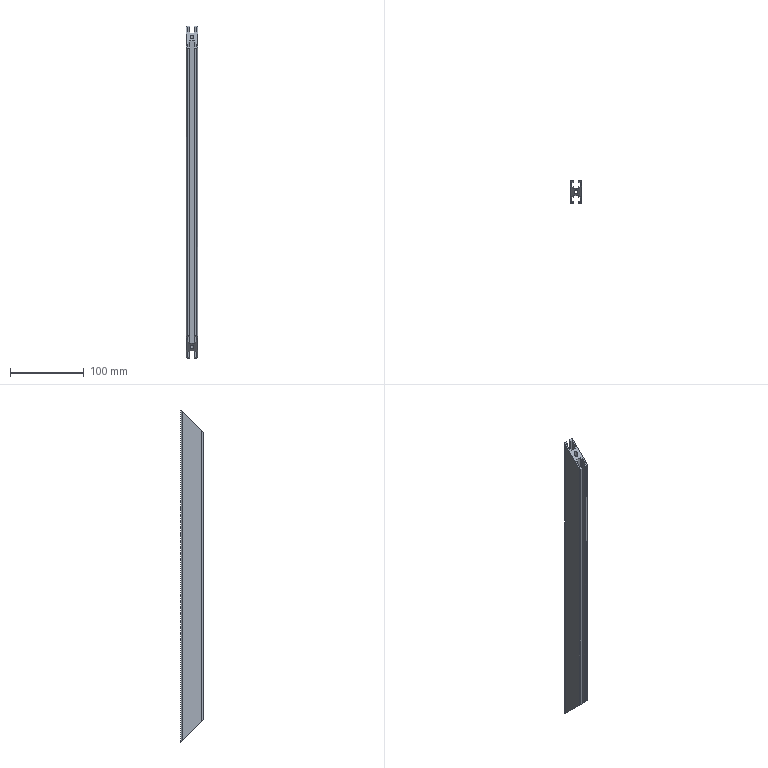Part | STEP file | OB1530-450 | 1 solid | 36 faces | box 15 x 30 x 450 mm | volume 102663 mm3 | plane 30 | cylinder 6 | commonest cylinder face diameters 3 x4 5 x2
STEP:
#1=CARTESIAN_POINT('',(2.5,0.,435.));
#2=VERTEX_POINT('',#1);
#3=CARTESIAN_POINT('',(-2.5,0.,435.));
#4=VERTEX_POINT('',#3);
#5=CARTESIAN_POINT('',(2.5,0.,435.));
#6=CARTESIAN_POINT('',(2.5,-5.,430.));
#7=CARTESIAN_POINT('',(-2.5,-5.,430.));
#8=CARTESIAN_POINT('',(-2.5,0.,435.));
#9=(BOUNDED_CURVE()B_SPLINE_CURVE(3,(#5,#6,#7,#8),.UNSPECIFIED.,.F.,.F.)B_SPLINE_CURVE_WITH_KNOTS((4,4),(4.712,7.854),.UNSPECIFIED.)CURVE()GEOMETRIC_REPRESENTATION_ITEM()RATIONAL_B_SPLINE_CURVE((1.,0.3333,0.3333,1.))REPRESENTATION_ITEM(''));
#10=EDGE_CURVE('',#2,#4,#9,.T.);
#11=ORIENTED_EDGE('',*,*,#10,.F.);
#12=CARTESIAN_POINT('',(2.5,0.,15.));
#13=VERTEX_POINT('',#12);
#14=CARTESIAN_POINT('',(2.5,0.,450.));
#15=DIRECTION('',(0.,0.,-1.));
#16=VECTOR('',#15,1000.);
#17=LINE('',#14,#16);
#18=EDGE_CURVE('',#2,#13,#17,.T.);
#19=ORIENTED_EDGE('',*,*,#18,.T.);
#20=CARTESIAN_POINT('',(-2.5,0.,15.));
#21=VERTEX_POINT('',#20);
#22=CARTESIAN_POINT('',(-2.5,0.,15.));
#23=CARTESIAN_POINT('',(-2.5,-5.,20.));
#24=CARTESIAN_POINT('',(2.5,-5.,20.));
#25=CARTESIAN_POINT('',(2.5,0.,15.));
#26=(BOUNDED_CURVE()B_SPLINE_CURVE(3,(#22,#23,#24,#25),.UNSPECIFIED.,.F.,.F.)B_SPLINE_CURVE_WITH_KNOTS((4,4),(1.571,4.712),.UNSPECIFIED.)CURVE()GEOMETRIC_REPRESENTATION_ITEM()RATIONAL_B_SPLINE_CURVE((1.,0.3333,0.3333,1.))REPRESENTATION_ITEM(''));
#27=EDGE_CURVE('',#21,#13,#26,.T.);
#28=ORIENTED_EDGE('',*,*,#27,.F.);
#29=CARTESIAN_POINT('',(-2.5,0.,450.));
#30=DIRECTION('',(0.,0.,-1.));
#31=VECTOR('',#30,1000.);
#32=LINE('',#29,#31);
#33=EDGE_CURVE('',#4,#21,#32,.T.);
#34=ORIENTED_EDGE('',*,*,#33,.F.);
#35=EDGE_LOOP('',(#11,#19,#28,#34));
#36=FACE_OUTER_BOUND('',#35,.T.);
#37=CARTESIAN_POINT('',(0.,0.,450.));
#38=DIRECTION('',(0.,0.,-1.));
#39=DIRECTION('',(-1.,0.,0.));
#40=AXIS2_PLACEMENT_3D('',#37,#38,#39);
#41=CYLINDRICAL_SURFACE('',#40,2.5);
#42=ADVANCED_FACE('',(#36),#41,.F.);
#43=CARTESIAN_POINT('',(6.,15.,450.));
#44=VERTEX_POINT('',#43);
#45=CARTESIAN_POINT('',(6.,15.,0.));
#46=VERTEX_POINT('',#45);
#47=CARTESIAN_POINT('',(6.,15.,450.));
#48=DIRECTION('',(0.,0.,-1.));
#49=VECTOR('',#48,1000.);
#50=LINE('',#47,#49);
#51=EDGE_CURVE('',#44,#46,#50,.T.);
#52=ORIENTED_EDGE('',*,*,#51,.F.);
#53=CARTESIAN_POINT('',(7.5,13.5,448.5));
#54=VERTEX_POINT('',#53);
#55=CARTESIAN_POINT('',(6.,15.,450.));
#56=CARTESIAN_POINT('',(6.879,15.,450.));
#57=CARTESIAN_POINT('',(7.5,14.379,449.379));
#58=CARTESIAN_POINT('',(7.5,13.5,448.5));
#59=(BOUNDED_CURVE()B_SPLINE_CURVE(3,(#55,#56,#57,#58),.UNSPECIFIED.,.F.,.F.)B_SPLINE_CURVE_WITH_KNOTS((4,4),(3.142,4.712),.UNSPECIFIED.)CURVE()GEOMETRIC_REPRESENTATION_ITEM()RATIONAL_B_SPLINE_CURVE((1.,0.8047,0.8047,1.))REPRESENTATION_ITEM(''));
#60=EDGE_CURVE('',#44,#54,#59,.T.);
#61=ORIENTED_EDGE('',*,*,#60,.T.);
#62=CARTESIAN_POINT('',(7.5,13.5,1.5));
#63=VERTEX_POINT('',#62);
#64=CARTESIAN_POINT('',(7.5,13.5,450.));
#65=DIRECTION('',(0.,0.,-1.));
#66=VECTOR('',#65,1000.);
#67=LINE('',#64,#66);
#68=EDGE_CURVE('',#54,#63,#67,.T.);
#69=ORIENTED_EDGE('',*,*,#68,.T.);
#70=CARTESIAN_POINT('',(7.5,13.5,1.5));
#71=CARTESIAN_POINT('',(7.5,14.379,0.6213));
#72=CARTESIAN_POINT('',(6.879,15.,0.));
#73=CARTESIAN_POINT('',(6.,15.,0.));
#74=(BOUNDED_CURVE()B_SPLINE_CURVE(3,(#70,#71,#72,#73),.UNSPECIFIED.,.F.,.F.)B_SPLINE_CURVE_WITH_KNOTS((4,4),(4.712,6.283),.UNSPECIFIED.)CURVE()GEOMETRIC_REPRESENTATION_ITEM()RATIONAL_B_SPLINE_CURVE((1.,0.8047,0.8047,1.))REPRESENTATION_ITEM(''));
#75=EDGE_CURVE('',#63,#46,#74,.T.);
#76=ORIENTED_EDGE('',*,*,#75,.T.);
#77=EDGE_LOOP('',(#52,#61,#69,#76));
#78=FACE_OUTER_BOUND('',#77,.T.);
#79=CARTESIAN_POINT('',(6.,13.5,450.));
#80=DIRECTION('',(0.,0.,-1.));
#81=DIRECTION('',(-1.,0.,0.));
#82=AXIS2_PLACEMENT_3D('',#79,#80,#81);
#83=CYLINDRICAL_SURFACE('',#82,1.5);
#84=ADVANCED_FACE('',(#78),#83,.T.);
#85=CARTESIAN_POINT('',(3.25,15.,0.));
#86=VERTEX_POINT('',#85);
#87=CARTESIAN_POINT('',(6.,15.,0.));
#88=DIRECTION('',(-1.,0.,0.));
#89=VECTOR('',#88,1000.);
#90=LINE('',#87,#89);
#91=EDGE_CURVE('',#46,#86,#90,.T.);
#92=ORIENTED_EDGE('',*,*,#91,.T.);
#93=CARTESIAN_POINT('',(3.25,15.,450.));
#94=VERTEX_POINT('',#93);
#95=CARTESIAN_POINT('',(3.25,15.,450.));
#96=DIRECTION('',(0.,0.,-1.));
#97=VECTOR('',#96,1000.);
#98=LINE('',#95,#97);
#99=EDGE_CURVE('',#94,#86,#98,.T.);
#100=ORIENTED_EDGE('',*,*,#99,.F.);
#101=CARTESIAN_POINT('',(6.,15.,450.));
#102=DIRECTION('',(-1.,0.,0.));
#103=VECTOR('',#102,1000.);
#104=LINE('',#101,#103);
#105=EDGE_CURVE('',#44,#94,#104,.T.);
#106=ORIENTED_EDGE('',*,*,#105,.F.);
#107=ORIENTED_EDGE('',*,*,#51,.T.);
#108=EDGE_LOOP('',(#92,#100,#106,#107));
#109=FACE_OUTER_BOUND('',#108,.T.);
#110=CARTESIAN_POINT('',(6.,15.,450.));
#111=DIRECTION('',(0.,-1.,0.));
#112=DIRECTION('',(0.,0.,-1.));
#113=AXIS2_PLACEMENT_3D('',#110,#111,#112);
#114=PLANE('',#113);
#115=ADVANCED_FACE('',(#109),#114,.F.);
#116=CARTESIAN_POINT('',(3.25,13.,448.));
#117=VERTEX_POINT('',#116);
#118=CARTESIAN_POINT('',(3.25,13.,2.));
#119=VERTEX_POINT('',#118);
#120=CARTESIAN_POINT('',(3.25,13.,450.));
#121=DIRECTION('',(0.,0.,-1.));
#122=VECTOR('',#121,1000.);
#123=LINE('',#120,#122);
#124=EDGE_CURVE('',#117,#119,#123,.T.);
#125=ORIENTED_EDGE('',*,*,#124,.F.);
#126=CARTESIAN_POINT('',(3.25,15.,450.));
#127=DIRECTION('',(0.,0.7071,0.7071));
#128=VECTOR('',#127,1000.);
#129=LINE('',#126,#128);
#130=EDGE_CURVE('',#117,#94,#129,.T.);
#131=ORIENTED_EDGE('',*,*,#130,.T.);
#132=ORIENTED_EDGE('',*,*,#99,.T.);
#133=CARTESIAN_POINT('',(3.25,-210.,225.));
#134=DIRECTION('',(0.,-0.7071,0.7071));
#135=VECTOR('',#134,1000.);
#136=LINE('',#133,#135);
#137=EDGE_CURVE('',#86,#119,#136,.T.);
#138=ORIENTED_EDGE('',*,*,#137,.T.);
#139=EDGE_LOOP('',(#125,#131,#132,#138));
#140=FACE_OUTER_BOUND('',#139,.T.);
#141=CARTESIAN_POINT('',(3.25,15.,450.));
#142=DIRECTION('',(1.,0.,0.));
#143=DIRECTION('',(0.,0.,-1.));
#144=AXIS2_PLACEMENT_3D('',#141,#142,#143);
#145=PLANE('',#144);
#146=ADVANCED_FACE('',(#140),#145,.F.);
#147=CARTESIAN_POINT('',(5.5,13.,448.));
#148=VERTEX_POINT('',#147);
#149=CARTESIAN_POINT('',(5.5,13.,2.));
#150=VERTEX_POINT('',#149);
#151=CARTESIAN_POINT('',(5.5,13.,450.));
#152=DIRECTION('',(0.,0.,-1.));
#153=VECTOR('',#152,1000.);
#154=LINE('',#151,#153);
#155=EDGE_CURVE('',#148,#150,#154,.T.);
#156=ORIENTED_EDGE('',*,*,#155,.F.);
#157=CARTESIAN_POINT('',(3.25,13.,448.));
#158=DIRECTION('',(-1.,0.,0.));
#159=VECTOR('',#158,1000.);
#160=LINE('',#157,#159);
#161=EDGE_CURVE('',#148,#117,#160,.T.);
#162=ORIENTED_EDGE('',*,*,#161,.T.);
#163=ORIENTED_EDGE('',*,*,#124,.T.);
#164=CARTESIAN_POINT('',(3.25,13.,2.));
#165=DIRECTION('',(1.,0.,0.));
#166=VECTOR('',#165,1000.);
#167=LINE('',#164,#166);
#168=EDGE_CURVE('',#119,#150,#167,.T.);
#169=ORIENTED_EDGE('',*,*,#168,.T.);
#170=EDGE_LOOP('',(#156,#162,#163,#169));
#171=FACE_OUTER_BOUND('',#170,.T.);
#172=CARTESIAN_POINT('',(3.25,13.,450.));
#173=DIRECTION('',(0.,1.,0.));
#174=DIRECTION('',(0.,0.,1.));
#175=AXIS2_PLACEMENT_3D('',#172,#173,#174);
#176=PLANE('',#175);
#177=ADVANCED_FACE('',(#171),#176,.F.);
#178=CARTESIAN_POINT('',(5.5,7.,442.));
#179=VERTEX_POINT('',#178);
#180=CARTESIAN_POINT('',(5.5,7.,8.));
#181=VERTEX_POINT('',#180);
#182=CARTESIAN_POINT('',(5.5,7.,450.));
#183=DIRECTION('',(0.,0.,-1.));
#184=VECTOR('',#183,1000.);
#185=LINE('',#182,#184);
#186=EDGE_CURVE('',#179,#181,#185,.T.);
#187=ORIENTED_EDGE('',*,*,#186,.F.);
#188=CARTESIAN_POINT('',(5.5,14.,449.));
#189=DIRECTION('',(0.,0.7071,0.7071));
#190=VECTOR('',#189,1000.);
#191=LINE('',#188,#190);
#192=EDGE_CURVE('',#179,#148,#191,.T.);
#193=ORIENTED_EDGE('',*,*,#192,.T.);
#194=ORIENTED_EDGE('',*,*,#155,.T.);
#195=CARTESIAN_POINT('',(5.5,-211.,226.));
#196=DIRECTION('',(0.,-0.7071,0.7071));
#197=VECTOR('',#196,1000.);
#198=LINE('',#195,#197);
#199=EDGE_CURVE('',#150,#181,#198,.T.);
#200=ORIENTED_EDGE('',*,*,#199,.T.);
#201=EDGE_LOOP('',(#187,#193,#194,#200));
#202=FACE_OUTER_BOUND('',#201,.T.);
#203=CARTESIAN_POINT('',(5.5,13.,450.));
#204=DIRECTION('',(1.,0.,0.));
#205=DIRECTION('',(0.,1.,0.));
#206=AXIS2_PLACEMENT_3D('',#203,#204,#205);
#207=PLANE('',#206);
#208=ADVANCED_FACE('',(#202),#207,.F.);
#209=CARTESIAN_POINT('',(3.25,7.,442.));
#210=VERTEX_POINT('',#209);
#211=CARTESIAN_POINT('',(3.25,7.,8.));
#212=VERTEX_POINT('',#211);
#213=CARTESIAN_POINT('',(3.25,7.,450.));
#214=DIRECTION('',(0.,0.,-1.));
#215=VECTOR('',#214,1000.);
#216=LINE('',#213,#215);
#217=EDGE_CURVE('',#210,#212,#216,.T.);
#218=ORIENTED_EDGE('',*,*,#217,.F.);
#219=CARTESIAN_POINT('',(5.5,7.,442.));
#220=DIRECTION('',(1.,0.,0.));
#221=VECTOR('',#220,1000.);
#222=LINE('',#219,#221);
#223=EDGE_CURVE('',#210,#179,#222,.T.);
#224=ORIENTED_EDGE('',*,*,#223,.T.);
#225=ORIENTED_EDGE('',*,*,#186,.T.);
#226=CARTESIAN_POINT('',(5.5,7.,8.));
#227=DIRECTION('',(-1.,0.,0.));
#228=VECTOR('',#227,1000.);
#229=LINE('',#226,#228);
#230=EDGE_CURVE('',#181,#212,#229,.T.);
#231=ORIENTED_EDGE('',*,*,#230,.T.);
#232=EDGE_LOOP('',(#218,#224,#225,#231));
#233=FACE_OUTER_BOUND('',#232,.T.);
#234=CARTESIAN_POINT('',(5.5,7.,450.));
#235=DIRECTION('',(0.,-1.,0.));
#236=DIRECTION('',(1.,0.,0.));
#237=AXIS2_PLACEMENT_3D('',#234,#235,#236);
#238=PLANE('',#237);
#239=ADVANCED_FACE('',(#233),#238,.F.);
#240=CARTESIAN_POINT('',(3.25,5.,440.));
#241=VERTEX_POINT('',#240);
#242=CARTESIAN_POINT('',(3.25,5.,10.));
#243=VERTEX_POINT('',#242);
#244=CARTESIAN_POINT('',(3.25,5.,450.));
#245=DIRECTION('',(0.,0.,-1.));
#246=VECTOR('',#245,1000.);
#247=LINE('',#244,#246);
#248=EDGE_CURVE('',#241,#243,#247,.T.);
#249=ORIENTED_EDGE('',*,*,#248,.F.);
#250=CARTESIAN_POINT('',(3.25,11.,446.));
#251=DIRECTION('',(0.,0.7071,0.7071));
#252=VECTOR('',#251,1000.);
#253=LINE('',#250,#252);
#254=EDGE_CURVE('',#241,#210,#253,.T.);
#255=ORIENTED_EDGE('',*,*,#254,.T.);
#256=ORIENTED_EDGE('',*,*,#217,.T.);
#257=CARTESIAN_POINT('',(3.25,-214.,229.));
#258=DIRECTION('',(0.,-0.7071,0.7071));
#259=VECTOR('',#258,1000.);
#260=LINE('',#257,#259);
#261=EDGE_CURVE('',#212,#243,#260,.T.);
#262=ORIENTED_EDGE('',*,*,#261,.T.);
#263=EDGE_LOOP('',(#249,#255,#256,#262));
#264=FACE_OUTER_BOUND('',#263,.T.);
#265=CARTESIAN_POINT('',(3.25,7.,450.));
#266=DIRECTION('',(1.,0.,0.));
#267=DIRECTION('',(0.,1.,0.));
#268=AXIS2_PLACEMENT_3D('',#265,#266,#267);
#269=PLANE('',#268);
#270=ADVANCED_FACE('',(#264),#269,.F.);
#271=CARTESIAN_POINT('',(-3.25,5.,440.));
#272=VERTEX_POINT('',#271);
#273=CARTESIAN_POINT('',(-3.25,5.,10.));
#274=VERTEX_POINT('',#273);
#275=CARTESIAN_POINT('',(-3.25,5.,450.));
#276=DIRECTION('',(0.,0.,-1.));
#277=VECTOR('',#276,1000.);
#278=LINE('',#275,#277);
#279=EDGE_CURVE('',#272,#274,#278,.T.);
#280=ORIENTED_EDGE('',*,*,#279,.F.);
#281=CARTESIAN_POINT('',(3.25,5.,440.));
#282=DIRECTION('',(1.,0.,0.));
#283=VECTOR('',#282,1000.);
#284=LINE('',#281,#283);
#285=EDGE_CURVE('',#272,#241,#284,.T.);
#286=ORIENTED_EDGE('',*,*,#285,.T.);
#287=ORIENTED_EDGE('',*,*,#248,.T.);
#288=CARTESIAN_POINT('',(3.25,5.,10.));
#289=DIRECTION('',(-1.,0.,0.));
#290=VECTOR('',#289,1000.);
#291=LINE('',#288,#290);
#292=EDGE_CURVE('',#243,#274,#291,.T.);
#293=ORIENTED_EDGE('',*,*,#292,.T.);
#294=EDGE_LOOP('',(#280,#286,#287,#293));
#295=FACE_OUTER_BOUND('',#294,.T.);
#296=CARTESIAN_POINT('',(3.25,5.,450.));
#297=DIRECTION('',(0.,-1.,0.));
#298=DIRECTION('',(0.,0.,-1.));
#299=AXIS2_PLACEMENT_3D('',#296,#297,#298);
#300=PLANE('',#299);
#301=ADVANCED_FACE('',(#295),#300,.F.);
#302=CARTESIAN_POINT('',(-3.25,7.,442.));
#303=VERTEX_POINT('',#302);
#304=CARTESIAN_POINT('',(-3.25,7.,8.));
#305=VERTEX_POINT('',#304);
#306=CARTESIAN_POINT('',(-3.25,7.,450.));
#307=DIRECTION('',(0.,0.,-1.));
#308=VECTOR('',#307,1000.);
#309=LINE('',#306,#308);
#310=EDGE_CURVE('',#303,#305,#309,.T.);
#311=ORIENTED_EDGE('',*,*,#310,.F.);
#312=CARTESIAN_POINT('',(-3.25,11.,446.));
#313=DIRECTION('',(0.,-0.7071,-0.7071));
#314=VECTOR('',#313,1000.);
#315=LINE('',#312,#314);
#316=EDGE_CURVE('',#303,#272,#315,.T.);
#317=ORIENTED_EDGE('',*,*,#316,.T.);
#318=ORIENTED_EDGE('',*,*,#279,.T.);
#319=CARTESIAN_POINT('',(-3.25,-214.,229.));
#320=DIRECTION('',(0.,0.7071,-0.7071));
#321=VECTOR('',#320,1000.);
#322=LINE('',#319,#321);
#323=EDGE_CURVE('',#274,#305,#322,.T.);
#324=ORIENTED_EDGE('',*,*,#323,.T.);
#325=EDGE_LOOP('',(#311,#317,#318,#324));
#326=FACE_OUTER_BOUND('',#325,.T.);
#327=CARTESIAN_POINT('',(-3.25,7.,450.));
#328=DIRECTION('',(-1.,0.,0.));
#329=DIRECTION('',(0.,-1.,0.));
#330=AXIS2_PLACEMENT_3D('',#327,#328,#329);
#331=PLANE('',#330);
#332=ADVANCED_FACE('',(#326),#331,.F.);
#333=CARTESIAN_POINT('',(-5.5,7.,442.));
#334=VERTEX_POINT('',#333);
#335=CARTESIAN_POINT('',(-5.5,7.,8.));
#336=VERTEX_POINT('',#335);
#337=CARTESIAN_POINT('',(-5.5,7.,450.));
#338=DIRECTION('',(0.,0.,-1.));
#339=VECTOR('',#338,1000.);
#340=LINE('',#337,#339);
#341=EDGE_CURVE('',#334,#336,#340,.T.);
#342=ORIENTED_EDGE('',*,*,#341,.F.);
#343=CARTESIAN_POINT('',(-5.5,7.,442.));
#344=DIRECTION('',(1.,0.,0.));
#345=VECTOR('',#344,1000.);
#346=LINE('',#343,#345);
#347=EDGE_CURVE('',#334,#303,#346,.T.);
#348=ORIENTED_EDGE('',*,*,#347,.T.);
#349=ORIENTED_EDGE('',*,*,#310,.T.);
#350=CARTESIAN_POINT('',(-5.5,7.,8.));
#351=DIRECTION('',(-1.,0.,0.));
#352=VECTOR('',#351,1000.);
#353=LINE('',#350,#352);
#354=EDGE_CURVE('',#305,#336,#353,.T.);
#355=ORIENTED_EDGE('',*,*,#354,.T.);
#356=EDGE_LOOP('',(#342,#348,#349,#355));
#357=FACE_OUTER_BOUND('',#356,.T.);
#358=CARTESIAN_POINT('',(-5.5,7.,450.));
#359=DIRECTION('',(0.,-1.,0.));
#360=DIRECTION('',(1.,0.,0.));
#361=AXIS2_PLACEMENT_3D('',#358,#359,#360);
#362=PLANE('',#361);
#363=ADVANCED_FACE('',(#357),#362,.F.);
#364=CARTESIAN_POINT('',(-5.5,13.,448.));
#365=VERTEX_POINT('',#364);
#366=CARTESIAN_POINT('',(-5.5,13.,2.));
#367=VERTEX_POINT('',#366);
#368=CARTESIAN_POINT('',(-5.5,13.,450.));
#369=DIRECTION('',(0.,0.,-1.));
#370=VECTOR('',#369,1000.);
#371=LINE('',#368,#370);
#372=EDGE_CURVE('',#365,#367,#371,.T.);
#373=ORIENTED_EDGE('',*,*,#372,.F.);
#374=CARTESIAN_POINT('',(-5.5,14.,449.));
#375=DIRECTION('',(0.,-0.7071,-0.7071));
#376=VECTOR('',#375,1000.);
#377=LINE('',#374,#376);
#378=EDGE_CURVE('',#365,#334,#377,.T.);
#379=ORIENTED_EDGE('',*,*,#378,.T.);
#380=ORIENTED_EDGE('',*,*,#341,.T.);
#381=CARTESIAN_POINT('',(-5.5,-211.,226.));
#382=DIRECTION('',(0.,0.7071,-0.7071));
#383=VECTOR('',#382,1000.);
#384=LINE('',#381,#383);
#385=EDGE_CURVE('',#336,#367,#384,.T.);
#386=ORIENTED_EDGE('',*,*,#385,.T.);
#387=EDGE_LOOP('',(#373,#379,#380,#386));
#388=FACE_OUTER_BOUND('',#387,.T.);
#389=CARTESIAN_POINT('',(-5.5,13.,450.));
#390=DIRECTION('',(-1.,0.,0.));
#391=DIRECTION('',(0.,-1.,0.));
#392=AXIS2_PLACEMENT_3D('',#389,#390,#391);
#393=PLANE('',#392);
#394=ADVANCED_FACE('',(#388),#393,.F.);
#395=CARTESIAN_POINT('',(-3.25,13.,448.));
#396=VERTEX_POINT('',#395);
#397=CARTESIAN_POINT('',(-3.25,13.,2.));
#398=VERTEX_POINT('',#397);
#399=CARTESIAN_POINT('',(-3.25,13.,450.));
#400=DIRECTION('',(0.,0.,-1.));
#401=VECTOR('',#400,1000.);
#402=LINE('',#399,#401);
#403=EDGE_CURVE('',#396,#398,#402,.T.);
#404=ORIENTED_EDGE('',*,*,#403,.F.);
#405=CARTESIAN_POINT('',(-3.25,13.,448.));
#406=DIRECTION('',(-1.,0.,0.));
#407=VECTOR('',#406,1000.);
#408=LINE('',#405,#407);
#409=EDGE_CURVE('',#396,#365,#408,.T.);
#410=ORIENTED_EDGE('',*,*,#409,.T.);
#411=ORIENTED_EDGE('',*,*,#372,.T.);
#412=CARTESIAN_POINT('',(-3.25,13.,2.));
#413=DIRECTION('',(1.,0.,0.));
#414=VECTOR('',#413,1000.);
#415=LINE('',#412,#414);
#416=EDGE_CURVE('',#367,#398,#415,.T.);
#417=ORIENTED_EDGE('',*,*,#416,.T.);
#418=EDGE_LOOP('',(#404,#410,#411,#417));
#419=FACE_OUTER_BOUND('',#418,.T.);
#420=CARTESIAN_POINT('',(-3.25,13.,450.));
#421=DIRECTION('',(0.,1.,0.));
#422=DIRECTION('',(0.,0.,1.));
#423=AXIS2_PLACEMENT_3D('',#420,#421,#422);
#424=PLANE('',#423);
#425=ADVANCED_FACE('',(#419),#424,.F.);
#426=CARTESIAN_POINT('',(-3.25,15.,450.));
#427=VERTEX_POINT('',#426);
#428=CARTESIAN_POINT('',(-3.25,15.,0.));
#429=VERTEX_POINT('',#428);
#430=CARTESIAN_POINT('',(-3.25,15.,450.));
#431=DIRECTION('',(0.,0.,-1.));
#432=VECTOR('',#431,1000.);
#433=LINE('',#430,#432);
#434=EDGE_CURVE('',#427,#429,#433,.T.);
#435=ORIENTED_EDGE('',*,*,#434,.F.);
#436=CARTESIAN_POINT('',(-3.25,15.,450.));
#437=DIRECTION('',(0.,-0.7071,-0.7071));
#438=VECTOR('',#437,1000.);
#439=LINE('',#436,#438);
#440=EDGE_CURVE('',#427,#396,#439,.T.);
#441=ORIENTED_EDGE('',*,*,#440,.T.);
#442=ORIENTED_EDGE('',*,*,#403,.T.);
#443=CARTESIAN_POINT('',(-3.25,-210.,225.));
#444=DIRECTION('',(0.,0.7071,-0.7071));
#445=VECTOR('',#444,1000.);
#446=LINE('',#443,#445);
#447=EDGE_CURVE('',#398,#429,#446,.T.);
#448=ORIENTED_EDGE('',*,*,#447,.T.);
#449=EDGE_LOOP('',(#435,#441,#442,#448));
#450=FACE_OUTER_BOUND('',#449,.T.);
#451=CARTESIAN_POINT('',(-3.25,15.,450.));
#452=DIRECTION('',(-1.,0.,0.));
#453=DIRECTION('',(0.,0.,1.));
#454=AXIS2_PLACEMENT_3D('',#451,#452,#453);
#455=PLANE('',#454);
#456=ADVANCED_FACE('',(#450),#455,.F.);
#457=CARTESIAN_POINT('',(-6.,15.,0.));
#458=VERTEX_POINT('',#457);
#459=CARTESIAN_POINT('',(-6.,15.,0.));
#460=DIRECTION('',(-1.,0.,0.));
#461=VECTOR('',#460,1000.);
#462=LINE('',#459,#461);
#463=EDGE_CURVE('',#429,#458,#462,.T.);
#464=ORIENTED_EDGE('',*,*,#463,.T.);
#465=CARTESIAN_POINT('',(-6.,15.,450.));
#466=VERTEX_POINT('',#465);
#467=CARTESIAN_POINT('',(-6.,15.,450.));
#468=DIRECTION('',(0.,0.,-1.));
#469=VECTOR('',#468,1000.);
#470=LINE('',#467,#469);
#471=EDGE_CURVE('',#466,#458,#470,.T.);
#472=ORIENTED_EDGE('',*,*,#471,.F.);
#473=CARTESIAN_POINT('',(-6.,15.,450.));
#474=DIRECTION('',(-1.,0.,0.));
#475=VECTOR('',#474,1000.);
#476=LINE('',#473,#475);
#477=EDGE_CURVE('',#427,#466,#476,.T.);
#478=ORIENTED_EDGE('',*,*,#477,.F.);
#479=ORIENTED_EDGE('',*,*,#434,.T.);
#480=EDGE_LOOP('',(#464,#472,#478,#479));
#481=FACE_OUTER_BOUND('',#480,.T.);
#482=CARTESIAN_POINT('',(-6.,15.,450.));
#483=DIRECTION('',(0.,-1.,0.));
#484=DIRECTION('',(0.,0.,-1.));
#485=AXIS2_PLACEMENT_3D('',#482,#483,#484);
#486=PLANE('',#485);
#487=ADVANCED_FACE('',(#481),#486,.F.);
#488=CARTESIAN_POINT('',(-7.5,13.5,448.5));
#489=VERTEX_POINT('',#488);
#490=CARTESIAN_POINT('',(-7.5,13.5,1.5));
#491=VERTEX_POINT('',#490);
#492=CARTESIAN_POINT('',(-7.5,13.5,450.));
#493=DIRECTION('',(0.,0.,-1.));
#494=VECTOR('',#493,1000.);
#495=LINE('',#492,#494);
#496=EDGE_CURVE('',#489,#491,#495,.T.);
#497=ORIENTED_EDGE('',*,*,#496,.F.);
#498=CARTESIAN_POINT('',(-7.5,13.5,448.5));
#499=CARTESIAN_POINT('',(-7.5,14.379,449.379));
#500=CARTESIAN_POINT('',(-6.879,15.,450.));
#501=CARTESIAN_POINT('',(-6.,15.,450.));
#502=(BOUNDED_CURVE()B_SPLINE_CURVE(3,(#498,#499,#500,#501),.UNSPECIFIED.,.F.,.F.)B_SPLINE_CURVE_WITH_KNOTS((4,4),(1.571,3.142),.UNSPECIFIED.)CURVE()GEOMETRIC_REPRESENTATION_ITEM()RATIONAL_B_SPLINE_CURVE((1.,0.8047,0.8047,1.))REPRESENTATION_ITEM(''));
#503=EDGE_CURVE('',#489,#466,#502,.T.);
#504=ORIENTED_EDGE('',*,*,#503,.T.);
#505=ORIENTED_EDGE('',*,*,#471,.T.);
#506=CARTESIAN_POINT('',(-6.,15.,0.));
#507=CARTESIAN_POINT('',(-6.879,15.,0.));
#508=CARTESIAN_POINT('',(-7.5,14.379,0.6213));
#509=CARTESIAN_POINT('',(-7.5,13.5,1.5));
#510=(BOUNDED_CURVE()B_SPLINE_CURVE(3,(#506,#507,#508,#509),.UNSPECIFIED.,.F.,.F.)B_SPLINE_CURVE_WITH_KNOTS((4,4),(0.,1.571),.UNSPECIFIED.)CURVE()GEOMETRIC_REPRESENTATION_ITEM()RATIONAL_B_SPLINE_CURVE((1.,0.8047,0.8047,1.))REPRESENTATION_ITEM(''));
#511=EDGE_CURVE('',#458,#491,#510,.T.);
#512=ORIENTED_EDGE('',*,*,#511,.T.);
#513=EDGE_LOOP('',(#497,#504,#505,#512));
#514=FACE_OUTER_BOUND('',#513,.T.);
#515=CARTESIAN_POINT('',(-6.,13.5,450.));
#516=DIRECTION('',(0.,0.,-1.));
#517=DIRECTION('',(-1.,0.,0.));
#518=AXIS2_PLACEMENT_3D('',#515,#516,#517);
#519=CYLINDRICAL_SURFACE('',#518,1.5);
#520=ADVANCED_FACE('',(#514),#519,.T.);
#521=CARTESIAN_POINT('',(-7.5,-13.5,421.5));
#522=VERTEX_POINT('',#521);
#523=CARTESIAN_POINT('',(-7.5,-13.5,28.5));
#524=VERTEX_POINT('',#523);
#525=CARTESIAN_POINT('',(-7.5,-13.5,450.));
#526=DIRECTION('',(0.,0.,-1.));
#527=VECTOR('',#526,1000.);
#528=LINE('',#525,#527);
#529=EDGE_CURVE('',#522,#524,#528,.T.);
#530=ORIENTED_EDGE('',*,*,#529,.F.);
#531=CARTESIAN_POINT('',(-7.5,-15.,420.));
#532=DIRECTION('',(0.,-0.7071,-0.7071));
#533=VECTOR('',#532,1000.);
#534=LINE('',#531,#533);
#535=EDGE_CURVE('',#489,#522,#534,.T.);
#536=ORIENTED_EDGE('',*,*,#535,.F.);
#537=ORIENTED_EDGE('',*,*,#496,.T.);
#538=CARTESIAN_POINT('',(-7.5,15.,0.));
#539=DIRECTION('',(0.,0.7071,-0.7071));
#540=VECTOR('',#539,1000.);
#541=LINE('',#538,#540);
#542=EDGE_CURVE('',#524,#491,#541,.T.);
#543=ORIENTED_EDGE('',*,*,#542,.F.);
#544=EDGE_LOOP('',(#530,#536,#537,#543));
#545=FACE_OUTER_BOUND('',#544,.T.);
#546=CARTESIAN_POINT('',(-7.5,-13.5,450.));
#547=DIRECTION('',(1.,0.,0.));
#548=DIRECTION('',(0.,0.,-1.));
#549=AXIS2_PLACEMENT_3D('',#546,#547,#548);
#550=PLANE('',#549);
#551=ADVANCED_FACE('',(#545),#550,.F.);
#552=CARTESIAN_POINT('',(-6.,-15.,420.));
#553=VERTEX_POINT('',#552);
#554=CARTESIAN_POINT('',(-6.,-15.,30.));
#555=VERTEX_POINT('',#554);
#556=CARTESIAN_POINT('',(-6.,-15.,450.));
#557=DIRECTION('',(0.,0.,-1.));
#558=VECTOR('',#557,1000.);
#559=LINE('',#556,#558);
#560=EDGE_CURVE('',#553,#555,#559,.T.);
#561=ORIENTED_EDGE('',*,*,#560,.F.);
#562=CARTESIAN_POINT('',(-6.,-15.,420.));
#563=CARTESIAN_POINT('',(-6.879,-15.,420.));
#564=CARTESIAN_POINT('',(-7.5,-14.379,420.621));
#565=CARTESIAN_POINT('',(-7.5,-13.5,421.5));
#566=(BOUNDED_CURVE()B_SPLINE_CURVE(3,(#562,#563,#564,#565),.UNSPECIFIED.,.F.,.F.)B_SPLINE_CURVE_WITH_KNOTS((4,4),(0.,1.571),.UNSPECIFIED.)CURVE()GEOMETRIC_REPRESENTATION_ITEM()RATIONAL_B_SPLINE_CURVE((1.,0.8047,0.8047,1.))REPRESENTATION_ITEM(''));
#567=EDGE_CURVE('',#553,#522,#566,.T.);
#568=ORIENTED_EDGE('',*,*,#567,.T.);
#569=ORIENTED_EDGE('',*,*,#529,.T.);
#570=CARTESIAN_POINT('',(-7.5,-13.5,28.5));
#571=CARTESIAN_POINT('',(-7.5,-14.379,29.379));
#572=CARTESIAN_POINT('',(-6.879,-15.,30.));
#573=CARTESIAN_POINT('',(-6.,-15.,30.));
#574=(BOUNDED_CURVE()B_SPLINE_CURVE(3,(#570,#571,#572,#573),.UNSPECIFIED.,.F.,.F.)B_SPLINE_CURVE_WITH_KNOTS((4,4),(1.571,3.142),.UNSPECIFIED.)CURVE()GEOMETRIC_REPRESENTATION_ITEM()RATIONAL_B_SPLINE_CURVE((1.,0.8047,0.8047,1.))REPRESENTATION_ITEM(''));
#575=EDGE_CURVE('',#524,#555,#574,.T.);
#576=ORIENTED_EDGE('',*,*,#575,.T.);
#577=EDGE_LOOP('',(#561,#568,#569,#576));
#578=FACE_OUTER_BOUND('',#577,.T.);
#579=CARTESIAN_POINT('',(-6.,-13.5,450.));
#580=DIRECTION('',(0.,0.,-1.));
#581=DIRECTION('',(-1.,0.,0.));
#582=AXIS2_PLACEMENT_3D('',#579,#580,#581);
#583=CYLINDRICAL_SURFACE('',#582,1.5);
#584=ADVANCED_FACE('',(#578),#583,.T.);
#585=CARTESIAN_POINT('',(-3.25,-15.,420.));
#586=VERTEX_POINT('',#585);
#587=CARTESIAN_POINT('',(-3.25,-15.,30.));
#588=VERTEX_POINT('',#587);
#589=CARTESIAN_POINT('',(-3.25,-15.,450.));
#590=DIRECTION('',(0.,0.,-1.));
#591=VECTOR('',#590,1000.);
#592=LINE('',#589,#591);
#593=EDGE_CURVE('',#586,#588,#592,.T.);
#594=ORIENTED_EDGE('',*,*,#593,.F.);
#595=CARTESIAN_POINT('',(7.5,-15.,420.));
#596=DIRECTION('',(-1.,0.,0.));
#597=VECTOR('',#596,1000.);
#598=LINE('',#595,#597);
#599=EDGE_CURVE('',#586,#553,#598,.T.);
#600=ORIENTED_EDGE('',*,*,#599,.T.);
#601=ORIENTED_EDGE('',*,*,#560,.T.);
#602=CARTESIAN_POINT('',(7.5,-15.,30.));
#603=DIRECTION('',(-1.,0.,0.));
#604=VECTOR('',#603,1000.);
#605=LINE('',#602,#604);
#606=EDGE_CURVE('',#588,#555,#605,.T.);
#607=ORIENTED_EDGE('',*,*,#606,.F.);
#608=EDGE_LOOP('',(#594,#600,#601,#607));
#609=FACE_OUTER_BOUND('',#608,.T.);
#610=CARTESIAN_POINT('',(-6.,-15.,450.));
#611=DIRECTION('',(0.,1.,0.));
#612=DIRECTION('',(0.,0.,1.));
#613=AXIS2_PLACEMENT_3D('',#610,#611,#612);
#614=PLANE('',#613);
#615=ADVANCED_FACE('',(#609),#614,.F.);
#616=CARTESIAN_POINT('',(-3.25,-13.,422.));
#617=VERTEX_POINT('',#616);
#618=CARTESIAN_POINT('',(-3.25,-13.,28.));
#619=VERTEX_POINT('',#618);
#620=CARTESIAN_POINT('',(-3.25,-13.,450.));
#621=DIRECTION('',(0.,0.,-1.));
#622=VECTOR('',#621,1000.);
#623=LINE('',#620,#622);
#624=EDGE_CURVE('',#617,#619,#623,.T.);
#625=ORIENTED_EDGE('',*,*,#624,.F.);
#626=CARTESIAN_POINT('',(-3.25,0.,435.));
#627=DIRECTION('',(0.,-0.7071,-0.7071));
#628=VECTOR('',#627,1000.);
#629=LINE('',#626,#628);
#630=EDGE_CURVE('',#617,#586,#629,.T.);
#631=ORIENTED_EDGE('',*,*,#630,.T.);
#632=ORIENTED_EDGE('',*,*,#593,.T.);
#633=CARTESIAN_POINT('',(-3.25,-225.,240.));
#634=DIRECTION('',(0.,0.7071,-0.7071));
#635=VECTOR('',#634,1000.);
#636=LINE('',#633,#635);
#637=EDGE_CURVE('',#588,#619,#636,.T.);
#638=ORIENTED_EDGE('',*,*,#637,.T.);
#639=EDGE_LOOP('',(#625,#631,#632,#638));
#640=FACE_OUTER_BOUND('',#639,.T.);
#641=CARTESIAN_POINT('',(-3.25,-15.,450.));
#642=DIRECTION('',(-1.,0.,0.));
#643=DIRECTION('',(0.,0.,1.));
#644=AXIS2_PLACEMENT_3D('',#641,#642,#643);
#645=PLANE('',#644);
#646=ADVANCED_FACE('',(#640),#645,.F.);
#647=CARTESIAN_POINT('',(-5.5,-13.,422.));
#648=VERTEX_POINT('',#647);
#649=CARTESIAN_POINT('',(-5.5,-13.,28.));
#650=VERTEX_POINT('',#649);
#651=CARTESIAN_POINT('',(-5.5,-13.,450.));
#652=DIRECTION('',(0.,0.,-1.));
#653=VECTOR('',#652,1000.);
#654=LINE('',#651,#653);
#655=EDGE_CURVE('',#648,#650,#654,.T.);
#656=ORIENTED_EDGE('',*,*,#655,.F.);
#657=CARTESIAN_POINT('',(-3.25,-13.,422.));
#658=DIRECTION('',(1.,0.,0.));
#659=VECTOR('',#658,1000.);
#660=LINE('',#657,#659);
#661=EDGE_CURVE('',#648,#617,#660,.T.);
#662=ORIENTED_EDGE('',*,*,#661,.T.);
#663=ORIENTED_EDGE('',*,*,#624,.T.);
#664=CARTESIAN_POINT('',(-3.25,-13.,28.));
#665=DIRECTION('',(-1.,0.,0.));
#666=VECTOR('',#665,1000.);
#667=LINE('',#664,#666);
#668=EDGE_CURVE('',#619,#650,#667,.T.);
#669=ORIENTED_EDGE('',*,*,#668,.T.);
#670=EDGE_LOOP('',(#656,#662,#663,#669));
#671=FACE_OUTER_BOUND('',#670,.T.);
#672=CARTESIAN_POINT('',(-3.25,-13.,450.));
#673=DIRECTION('',(0.,-1.,0.));
#674=DIRECTION('',(0.,0.,-1.));
#675=AXIS2_PLACEMENT_3D('',#672,#673,#674);
#676=PLANE('',#675);
#677=ADVANCED_FACE('',(#671),#676,.F.);
#678=CARTESIAN_POINT('',(-5.5,-7.,428.));
#679=VERTEX_POINT('',#678);
#680=CARTESIAN_POINT('',(-5.5,-7.,22.));
#681=VERTEX_POINT('',#680);
#682=CARTESIAN_POINT('',(-5.5,-7.,450.));
#683=DIRECTION('',(0.,0.,-1.));
#684=VECTOR('',#683,1000.);
#685=LINE('',#682,#684);
#686=EDGE_CURVE('',#679,#681,#685,.T.);
#687=ORIENTED_EDGE('',*,*,#686,.F.);
#688=CARTESIAN_POINT('',(-5.5,1.,436.));
#689=DIRECTION('',(0.,-0.7071,-0.7071));
#690=VECTOR('',#689,1000.);
#691=LINE('',#688,#690);
#692=EDGE_CURVE('',#679,#648,#691,.T.);
#693=ORIENTED_EDGE('',*,*,#692,.T.);
#694=ORIENTED_EDGE('',*,*,#655,.T.);
#695=CARTESIAN_POINT('',(-5.5,-224.,239.));
#696=DIRECTION('',(0.,0.7071,-0.7071));
#697=VECTOR('',#696,1000.);
#698=LINE('',#695,#697);
#699=EDGE_CURVE('',#650,#681,#698,.T.);
#700=ORIENTED_EDGE('',*,*,#699,.T.);
#701=EDGE_LOOP('',(#687,#693,#694,#700));
#702=FACE_OUTER_BOUND('',#701,.T.);
#703=CARTESIAN_POINT('',(-5.5,-13.,450.));
#704=DIRECTION('',(-1.,0.,0.));
#705=DIRECTION('',(0.,-1.,0.));
#706=AXIS2_PLACEMENT_3D('',#703,#704,#705);
#707=PLANE('',#706);
#708=ADVANCED_FACE('',(#702),#707,.F.);
#709=CARTESIAN_POINT('',(-3.25,-7.,428.));
#710=VERTEX_POINT('',#709);
#711=CARTESIAN_POINT('',(-3.25,-7.,22.));
#712=VERTEX_POINT('',#711);
#713=CARTESIAN_POINT('',(-3.25,-7.,450.));
#714=DIRECTION('',(0.,0.,-1.));
#715=VECTOR('',#714,1000.);
#716=LINE('',#713,#715);
#717=EDGE_CURVE('',#710,#712,#716,.T.);
#718=ORIENTED_EDGE('',*,*,#717,.F.);
#719=CARTESIAN_POINT('',(-5.5,-7.,428.));
#720=DIRECTION('',(-1.,0.,0.));
#721=VECTOR('',#720,1000.);
#722=LINE('',#719,#721);
#723=EDGE_CURVE('',#710,#679,#722,.T.);
#724=ORIENTED_EDGE('',*,*,#723,.T.);
#725=ORIENTED_EDGE('',*,*,#686,.T.);
#726=CARTESIAN_POINT('',(-5.5,-7.,22.));
#727=DIRECTION('',(1.,0.,0.));
#728=VECTOR('',#727,1000.);
#729=LINE('',#726,#728);
#730=EDGE_CURVE('',#681,#712,#729,.T.);
#731=ORIENTED_EDGE('',*,*,#730,.T.);
#732=EDGE_LOOP('',(#718,#724,#725,#731));
#733=FACE_OUTER_BOUND('',#732,.T.);
#734=CARTESIAN_POINT('',(-5.5,-7.,450.));
#735=DIRECTION('',(0.,1.,0.));
#736=DIRECTION('',(-1.,0.,0.));
#737=AXIS2_PLACEMENT_3D('',#734,#735,#736);
#738=PLANE('',#737);
#739=ADVANCED_FACE('',(#733),#738,.F.);
#740=CARTESIAN_POINT('',(-3.25,-5.,430.));
#741=VERTEX_POINT('',#740);
#742=CARTESIAN_POINT('',(-3.25,-5.,20.));
#743=VERTEX_POINT('',#742);
#744=CARTESIAN_POINT('',(-3.25,-5.,450.));
#745=DIRECTION('',(0.,0.,-1.));
#746=VECTOR('',#745,1000.);
#747=LINE('',#744,#746);
#748=EDGE_CURVE('',#741,#743,#747,.T.);
#749=ORIENTED_EDGE('',*,*,#748,.F.);
#750=CARTESIAN_POINT('',(-3.25,4.,439.));
#751=DIRECTION('',(0.,-0.7071,-0.7071));
#752=VECTOR('',#751,1000.);
#753=LINE('',#750,#752);
#754=EDGE_CURVE('',#741,#710,#753,.T.);
#755=ORIENTED_EDGE('',*,*,#754,.T.);
#756=ORIENTED_EDGE('',*,*,#717,.T.);
#757=CARTESIAN_POINT('',(-3.25,-221.,236.));
#758=DIRECTION('',(0.,0.7071,-0.7071));
#759=VECTOR('',#758,1000.);
#760=LINE('',#757,#759);
#761=EDGE_CURVE('',#712,#743,#760,.T.);
#762=ORIENTED_EDGE('',*,*,#761,.T.);
#763=EDGE_LOOP('',(#749,#755,#756,#762));
#764=FACE_OUTER_BOUND('',#763,.T.);
#765=CARTESIAN_POINT('',(-3.25,-7.,450.));
#766=DIRECTION('',(-1.,0.,0.));
#767=DIRECTION('',(0.,-1.,0.));
#768=AXIS2_PLACEMENT_3D('',#765,#766,#767);
#769=PLANE('',#768);
#770=ADVANCED_FACE('',(#764),#769,.F.);
#771=CARTESIAN_POINT('',(3.25,-5.,430.));
#772=VERTEX_POINT('',#771);
#773=CARTESIAN_POINT('',(3.25,-5.,20.));
#774=VERTEX_POINT('',#773);
#775=CARTESIAN_POINT('',(3.25,-5.,450.));
#776=DIRECTION('',(0.,0.,-1.));
#777=VECTOR('',#776,1000.);
#778=LINE('',#775,#777);
#779=EDGE_CURVE('',#772,#774,#778,.T.);
#780=ORIENTED_EDGE('',*,*,#779,.F.);
#781=CARTESIAN_POINT('',(3.25,-5.,430.));
#782=DIRECTION('',(-1.,0.,0.));
#783=VECTOR('',#782,1000.);
#784=LINE('',#781,#783);
#785=EDGE_CURVE('',#772,#741,#784,.T.);
#786=ORIENTED_EDGE('',*,*,#785,.T.);
#787=ORIENTED_EDGE('',*,*,#748,.T.);
#788=CARTESIAN_POINT('',(3.25,-5.,20.));
#789=DIRECTION('',(1.,0.,0.));
#790=VECTOR('',#789,1000.);
#791=LINE('',#788,#790);
#792=EDGE_CURVE('',#743,#774,#791,.T.);
#793=ORIENTED_EDGE('',*,*,#792,.T.);
#794=EDGE_LOOP('',(#780,#786,#787,#793));
#795=FACE_OUTER_BOUND('',#794,.T.);
#796=CARTESIAN_POINT('',(3.25,-5.,450.));
#797=DIRECTION('',(0.,1.,0.));
#798=DIRECTION('',(0.,0.,1.));
#799=AXIS2_PLACEMENT_3D('',#796,#797,#798);
#800=PLANE('',#799);
#801=ADVANCED_FACE('',(#795),#800,.F.);
#802=CARTESIAN_POINT('',(3.25,-7.,428.));
#803=VERTEX_POINT('',#802);
#804=CARTESIAN_POINT('',(3.25,-7.,22.));
#805=VERTEX_POINT('',#804);
#806=CARTESIAN_POINT('',(3.25,-7.,450.));
#807=DIRECTION('',(0.,0.,-1.));
#808=VECTOR('',#807,1000.);
#809=LINE('',#806,#808);
#810=EDGE_CURVE('',#803,#805,#809,.T.);
#811=ORIENTED_EDGE('',*,*,#810,.F.);
#812=CARTESIAN_POINT('',(3.25,4.,439.));
#813=DIRECTION('',(0.,0.7071,0.7071));
#814=VECTOR('',#813,1000.);
#815=LINE('',#812,#814);
#816=EDGE_CURVE('',#803,#772,#815,.T.);
#817=ORIENTED_EDGE('',*,*,#816,.T.);
#818=ORIENTED_EDGE('',*,*,#779,.T.);
#819=CARTESIAN_POINT('',(3.25,-221.,236.));
#820=DIRECTION('',(0.,-0.7071,0.7071));
#821=VECTOR('',#820,1000.);
#822=LINE('',#819,#821);
#823=EDGE_CURVE('',#774,#805,#822,.T.);
#824=ORIENTED_EDGE('',*,*,#823,.T.);
#825=EDGE_LOOP('',(#811,#817,#818,#824));
#826=FACE_OUTER_BOUND('',#825,.T.);
#827=CARTESIAN_POINT('',(3.25,-7.,450.));
#828=DIRECTION('',(1.,0.,0.));
#829=DIRECTION('',(0.,1.,0.));
#830=AXIS2_PLACEMENT_3D('',#827,#828,#829);
#831=PLANE('',#830);
#832=ADVANCED_FACE('',(#826),#831,.F.);
#833=CARTESIAN_POINT('',(5.5,-7.,428.));
#834=VERTEX_POINT('',#833);
#835=CARTESIAN_POINT('',(5.5,-7.,22.));
#836=VERTEX_POINT('',#835);
#837=CARTESIAN_POINT('',(5.5,-7.,450.));
#838=DIRECTION('',(0.,0.,-1.));
#839=VECTOR('',#838,1000.);
#840=LINE('',#837,#839);
#841=EDGE_CURVE('',#834,#836,#840,.T.);
#842=ORIENTED_EDGE('',*,*,#841,.F.);
#843=CARTESIAN_POINT('',(5.5,-7.,428.));
#844=DIRECTION('',(-1.,0.,0.));
#845=VECTOR('',#844,1000.);
#846=LINE('',#843,#845);
#847=EDGE_CURVE('',#834,#803,#846,.T.);
#848=ORIENTED_EDGE('',*,*,#847,.T.);
#849=ORIENTED_EDGE('',*,*,#810,.T.);
#850=CARTESIAN_POINT('',(5.5,-7.,22.));
#851=DIRECTION('',(1.,0.,0.));
#852=VECTOR('',#851,1000.);
#853=LINE('',#850,#852);
#854=EDGE_CURVE('',#805,#836,#853,.T.);
#855=ORIENTED_EDGE('',*,*,#854,.T.);
#856=EDGE_LOOP('',(#842,#848,#849,#855));
#857=FACE_OUTER_BOUND('',#856,.T.);
#858=CARTESIAN_POINT('',(5.5,-7.,450.));
#859=DIRECTION('',(0.,1.,0.));
#860=DIRECTION('',(-1.,0.,0.));
#861=AXIS2_PLACEMENT_3D('',#858,#859,#860);
#862=PLANE('',#861);
#863=ADVANCED_FACE('',(#857),#862,.F.);
#864=CARTESIAN_POINT('',(5.5,-13.,422.));
#865=VERTEX_POINT('',#864);
#866=CARTESIAN_POINT('',(5.5,-13.,28.));
#867=VERTEX_POINT('',#866);
#868=CARTESIAN_POINT('',(5.5,-13.,450.));
#869=DIRECTION('',(0.,0.,-1.));
#870=VECTOR('',#869,1000.);
#871=LINE('',#868,#870);
#872=EDGE_CURVE('',#865,#867,#871,.T.);
#873=ORIENTED_EDGE('',*,*,#872,.F.);
#874=CARTESIAN_POINT('',(5.5,1.,436.));
#875=DIRECTION('',(0.,0.7071,0.7071));
#876=VECTOR('',#875,1000.);
#877=LINE('',#874,#876);
#878=EDGE_CURVE('',#865,#834,#877,.T.);
#879=ORIENTED_EDGE('',*,*,#878,.T.);
#880=ORIENTED_EDGE('',*,*,#841,.T.);
#881=CARTESIAN_POINT('',(5.5,-224.,239.));
#882=DIRECTION('',(0.,-0.7071,0.7071));
#883=VECTOR('',#882,1000.);
#884=LINE('',#881,#883);
#885=EDGE_CURVE('',#836,#867,#884,.T.);
#886=ORIENTED_EDGE('',*,*,#885,.T.);
#887=EDGE_LOOP('',(#873,#879,#880,#886));
#888=FACE_OUTER_BOUND('',#887,.T.);
#889=CARTESIAN_POINT('',(5.5,-13.,450.));
#890=DIRECTION('',(1.,0.,0.));
#891=DIRECTION('',(0.,1.,0.));
#892=AXIS2_PLACEMENT_3D('',#889,#890,#891);
#893=PLANE('',#892);
#894=ADVANCED_FACE('',(#888),#893,.F.);
#895=CARTESIAN_POINT('',(3.25,-13.,422.));
#896=VERTEX_POINT('',#895);
#897=CARTESIAN_POINT('',(3.25,-13.,28.));
#898=VERTEX_POINT('',#897);
#899=CARTESIAN_POINT('',(3.25,-13.,450.));
#900=DIRECTION('',(0.,0.,-1.));
#901=VECTOR('',#900,1000.);
#902=LINE('',#899,#901);
#903=EDGE_CURVE('',#896,#898,#902,.T.);
#904=ORIENTED_EDGE('',*,*,#903,.F.);
#905=CARTESIAN_POINT('',(3.25,-13.,422.));
#906=DIRECTION('',(1.,0.,0.));
#907=VECTOR('',#906,1000.);
#908=LINE('',#905,#907);
#909=EDGE_CURVE('',#896,#865,#908,.T.);
#910=ORIENTED_EDGE('',*,*,#909,.T.);
#911=ORIENTED_EDGE('',*,*,#872,.T.);
#912=CARTESIAN_POINT('',(3.25,-13.,28.));
#913=DIRECTION('',(-1.,0.,0.));
#914=VECTOR('',#913,1000.);
#915=LINE('',#912,#914);
#916=EDGE_CURVE('',#867,#898,#915,.T.);
#917=ORIENTED_EDGE('',*,*,#916,.T.);
#918=EDGE_LOOP('',(#904,#910,#911,#917));
#919=FACE_OUTER_BOUND('',#918,.T.);
#920=CARTESIAN_POINT('',(3.25,-13.,450.));
#921=DIRECTION('',(0.,-1.,0.));
#922=DIRECTION('',(0.,0.,-1.));
#923=AXIS2_PLACEMENT_3D('',#920,#921,#922);
#924=PLANE('',#923);
#925=ADVANCED_FACE('',(#919),#924,.F.);
#926=CARTESIAN_POINT('',(3.25,-15.,420.));
#927=VERTEX_POINT('',#926);
#928=CARTESIAN_POINT('',(3.25,-15.,30.));
#929=VERTEX_POINT('',#928);
#930=CARTESIAN_POINT('',(3.25,-15.,450.));
#931=DIRECTION('',(0.,0.,-1.));
#932=VECTOR('',#931,1000.);
#933=LINE('',#930,#932);
#934=EDGE_CURVE('',#927,#929,#933,.T.);
#935=ORIENTED_EDGE('',*,*,#934,.F.);
#936=CARTESIAN_POINT('',(3.25,0.,435.));
#937=DIRECTION('',(0.,0.7071,0.7071));
#938=VECTOR('',#937,1000.);
#939=LINE('',#936,#938);
#940=EDGE_CURVE('',#927,#896,#939,.T.);
#941=ORIENTED_EDGE('',*,*,#940,.T.);
#942=ORIENTED_EDGE('',*,*,#903,.T.);
#943=CARTESIAN_POINT('',(3.25,-225.,240.));
#944=DIRECTION('',(0.,-0.7071,0.7071));
#945=VECTOR('',#944,1000.);
#946=LINE('',#943,#945);
#947=EDGE_CURVE('',#898,#929,#946,.T.);
#948=ORIENTED_EDGE('',*,*,#947,.T.);
#949=EDGE_LOOP('',(#935,#941,#942,#948));
#950=FACE_OUTER_BOUND('',#949,.T.);
#951=CARTESIAN_POINT('',(3.25,-15.,450.));
#952=DIRECTION('',(1.,0.,0.));
#953=DIRECTION('',(0.,0.,-1.));
#954=AXIS2_PLACEMENT_3D('',#951,#952,#953);
#955=PLANE('',#954);
#956=ADVANCED_FACE('',(#950),#955,.F.);
#957=CARTESIAN_POINT('',(6.,-15.,420.));
#958=VERTEX_POINT('',#957);
#959=CARTESIAN_POINT('',(6.,-15.,30.));
#960=VERTEX_POINT('',#959);
#961=CARTESIAN_POINT('',(6.,-15.,450.));
#962=DIRECTION('',(0.,0.,-1.));
#963=VECTOR('',#962,1000.);
#964=LINE('',#961,#963);
#965=EDGE_CURVE('',#958,#960,#964,.T.);
#966=ORIENTED_EDGE('',*,*,#965,.F.);
#967=CARTESIAN_POINT('',(7.5,-15.,420.));
#968=DIRECTION('',(-1.,0.,0.));
#969=VECTOR('',#968,1000.);
#970=LINE('',#967,#969);
#971=EDGE_CURVE('',#958,#927,#970,.T.);
#972=ORIENTED_EDGE('',*,*,#971,.T.);
#973=ORIENTED_EDGE('',*,*,#934,.T.);
#974=CARTESIAN_POINT('',(7.5,-15.,30.));
#975=DIRECTION('',(-1.,0.,0.));
#976=VECTOR('',#975,1000.);
#977=LINE('',#974,#976);
#978=EDGE_CURVE('',#960,#929,#977,.T.);
#979=ORIENTED_EDGE('',*,*,#978,.F.);
#980=EDGE_LOOP('',(#966,#972,#973,#979));
#981=FACE_OUTER_BOUND('',#980,.T.);
#982=CARTESIAN_POINT('',(6.,-15.,450.));
#983=DIRECTION('',(0.,1.,0.));
#984=DIRECTION('',(0.,0.,1.));
#985=AXIS2_PLACEMENT_3D('',#982,#983,#984);
#986=PLANE('',#985);
#987=ADVANCED_FACE('',(#981),#986,.F.);
#988=CARTESIAN_POINT('',(7.5,-13.5,421.5));
#989=VERTEX_POINT('',#988);
#990=CARTESIAN_POINT('',(7.5,-13.5,28.5));
#991=VERTEX_POINT('',#990);
#992=CARTESIAN_POINT('',(7.5,-13.5,450.));
#993=DIRECTION('',(0.,0.,-1.));
#994=VECTOR('',#993,1000.);
#995=LINE('',#992,#994);
#996=EDGE_CURVE('',#989,#991,#995,.T.);
#997=ORIENTED_EDGE('',*,*,#996,.F.);
#998=CARTESIAN_POINT('',(7.5,-13.5,421.5));
#999=CARTESIAN_POINT('',(7.5,-14.379,420.621));
#1000=CARTESIAN_POINT('',(6.879,-15.,420.));
#1001=CARTESIAN_POINT('',(6.,-15.,420.));
#1002=(BOUNDED_CURVE()B_SPLINE_CURVE(3,(#998,#999,#1000,#1001),.UNSPECIFIED.,.F.,.F.)B_SPLINE_CURVE_WITH_KNOTS((4,4),(4.712,6.283),.UNSPECIFIED.)CURVE()GEOMETRIC_REPRESENTATION_ITEM()RATIONAL_B_SPLINE_CURVE((1.,0.8047,0.8047,1.))REPRESENTATION_ITEM(''));
#1003=EDGE_CURVE('',#989,#958,#1002,.T.);
#1004=ORIENTED_EDGE('',*,*,#1003,.T.);
#1005=ORIENTED_EDGE('',*,*,#965,.T.);
#1006=CARTESIAN_POINT('',(6.,-15.,30.));
#1007=CARTESIAN_POINT('',(6.879,-15.,30.));
#1008=CARTESIAN_POINT('',(7.5,-14.379,29.379));
#1009=CARTESIAN_POINT('',(7.5,-13.5,28.5));
#1010=(BOUNDED_CURVE()B_SPLINE_CURVE(3,(#1006,#1007,#1008,#1009),.UNSPECIFIED.,.F.,.F.)B_SPLINE_CURVE_WITH_KNOTS((4,4),(3.142,4.712),.UNSPECIFIED.)CURVE()GEOMETRIC_REPRESENTATION_ITEM()RATIONAL_B_SPLINE_CURVE((1.,0.8047,0.8047,1.))REPRESENTATION_ITEM(''));
#1011=EDGE_CURVE('',#960,#991,#1010,.T.);
#1012=ORIENTED_EDGE('',*,*,#1011,.T.);
#1013=EDGE_LOOP('',(#997,#1004,#1005,#1012));
#1014=FACE_OUTER_BOUND('',#1013,.T.);
#1015=CARTESIAN_POINT('',(6.,-13.5,450.));
#1016=DIRECTION('',(0.,0.,-1.));
#1017=DIRECTION('',(-1.,0.,0.));
#1018=AXIS2_PLACEMENT_3D('',#1015,#1016,#1017);
#1019=CYLINDRICAL_SURFACE('',#1018,1.5);
#1020=ADVANCED_FACE('',(#1014),#1019,.T.);
#1021=ORIENTED_EDGE('',*,*,#68,.F.);
#1022=CARTESIAN_POINT('',(7.5,-15.,420.));
#1023=DIRECTION('',(0.,-0.7071,-0.7071));
#1024=VECTOR('',#1023,1000.);
#1025=LINE('',#1022,#1024);
#1026=EDGE_CURVE('',#54,#989,#1025,.T.);
#1027=ORIENTED_EDGE('',*,*,#1026,.T.);
#1028=ORIENTED_EDGE('',*,*,#996,.T.);
#1029=CARTESIAN_POINT('',(7.5,15.,0.));
#1030=DIRECTION('',(0.,0.7071,-0.7071));
#1031=VECTOR('',#1030,1000.);
#1032=LINE('',#1029,#1031);
#1033=EDGE_CURVE('',#991,#63,#1032,.T.);
#1034=ORIENTED_EDGE('',*,*,#1033,.T.);
#1035=EDGE_LOOP('',(#1021,#1027,#1028,#1034));
#1036=FACE_OUTER_BOUND('',#1035,.T.);
#1037=CARTESIAN_POINT('',(7.5,-13.5,450.));
#1038=DIRECTION('',(-1.,0.,0.));
#1039=DIRECTION('',(0.,0.,1.));
#1040=AXIS2_PLACEMENT_3D('',#1037,#1038,#1039);
#1041=PLANE('',#1040);
#1042=ADVANCED_FACE('',(#1036),#1041,.F.);
#1043=ORIENTED_EDGE('',*,*,#18,.F.);
#1044=CARTESIAN_POINT('',(-2.5,0.,435.));
#1045=CARTESIAN_POINT('',(-2.5,5.,440.));
#1046=CARTESIAN_POINT('',(2.5,5.,440.));
#1047=CARTESIAN_POINT('',(2.5,0.,435.));
#1048=(BOUNDED_CURVE()B_SPLINE_CURVE(3,(#1044,#1045,#1046,#1047),.UNSPECIFIED.,.F.,.F.)B_SPLINE_CURVE_WITH_KNOTS((4,4),(1.571,4.712),.UNSPECIFIED.)CURVE()GEOMETRIC_REPRESENTATION_ITEM()RATIONAL_B_SPLINE_CURVE((1.,0.3333,0.3333,1.))REPRESENTATION_ITEM(''));
#1049=EDGE_CURVE('',#4,#2,#1048,.T.);
#1050=ORIENTED_EDGE('',*,*,#1049,.F.);
#1051=ORIENTED_EDGE('',*,*,#33,.T.);
#1052=CARTESIAN_POINT('',(2.5,0.,15.));
#1053=CARTESIAN_POINT('',(2.5,5.,10.));
#1054=CARTESIAN_POINT('',(-2.5,5.,10.));
#1055=CARTESIAN_POINT('',(-2.5,0.,15.));
#1056=(BOUNDED_CURVE()B_SPLINE_CURVE(3,(#1052,#1053,#1054,#1055),.UNSPECIFIED.,.F.,.F.)B_SPLINE_CURVE_WITH_KNOTS((4,4),(4.712,7.854),.UNSPECIFIED.)CURVE()GEOMETRIC_REPRESENTATION_ITEM()RATIONAL_B_SPLINE_CURVE((1.,0.3333,0.3333,1.))REPRESENTATION_ITEM(''));
#1057=EDGE_CURVE('',#13,#21,#1056,.T.);
#1058=ORIENTED_EDGE('',*,*,#1057,.F.);
#1059=EDGE_LOOP('',(#1043,#1050,#1051,#1058));
#1060=FACE_OUTER_BOUND('',#1059,.T.);
#1061=CARTESIAN_POINT('',(0.,0.,450.));
#1062=DIRECTION('',(0.,0.,-1.));
#1063=DIRECTION('',(-1.,0.,0.));
#1064=AXIS2_PLACEMENT_3D('',#1061,#1062,#1063);
#1065=CYLINDRICAL_SURFACE('',#1064,2.5);
#1066=ADVANCED_FACE('',(#1060),#1065,.F.);
#1067=ORIENTED_EDGE('',*,*,#27,.T.);
#1068=ORIENTED_EDGE('',*,*,#1057,.T.);
#1069=EDGE_LOOP('',(#1067,#1068));
#1070=FACE_BOUND('',#1069,.T.);
#1071=ORIENTED_EDGE('',*,*,#1033,.F.);
#1072=ORIENTED_EDGE('',*,*,#1011,.F.);
#1073=ORIENTED_EDGE('',*,*,#978,.T.);
#1074=ORIENTED_EDGE('',*,*,#947,.F.);
#1075=ORIENTED_EDGE('',*,*,#916,.F.);
#1076=ORIENTED_EDGE('',*,*,#885,.F.);
#1077=ORIENTED_EDGE('',*,*,#854,.F.);
#1078=ORIENTED_EDGE('',*,*,#823,.F.);
#1079=ORIENTED_EDGE('',*,*,#792,.F.);
#1080=ORIENTED_EDGE('',*,*,#761,.F.);
#1081=ORIENTED_EDGE('',*,*,#730,.F.);
#1082=ORIENTED_EDGE('',*,*,#699,.F.);
#1083=ORIENTED_EDGE('',*,*,#668,.F.);
#1084=ORIENTED_EDGE('',*,*,#637,.F.);
#1085=ORIENTED_EDGE('',*,*,#606,.T.);
#1086=ORIENTED_EDGE('',*,*,#575,.F.);
#1087=ORIENTED_EDGE('',*,*,#542,.T.);
#1088=ORIENTED_EDGE('',*,*,#511,.F.);
#1089=ORIENTED_EDGE('',*,*,#463,.F.);
#1090=ORIENTED_EDGE('',*,*,#447,.F.);
#1091=ORIENTED_EDGE('',*,*,#416,.F.);
#1092=ORIENTED_EDGE('',*,*,#385,.F.);
#1093=ORIENTED_EDGE('',*,*,#354,.F.);
#1094=ORIENTED_EDGE('',*,*,#323,.F.);
#1095=ORIENTED_EDGE('',*,*,#292,.F.);
#1096=ORIENTED_EDGE('',*,*,#261,.F.);
#1097=ORIENTED_EDGE('',*,*,#230,.F.);
#1098=ORIENTED_EDGE('',*,*,#199,.F.);
#1099=ORIENTED_EDGE('',*,*,#168,.F.);
#1100=ORIENTED_EDGE('',*,*,#137,.F.);
#1101=ORIENTED_EDGE('',*,*,#91,.F.);
#1102=ORIENTED_EDGE('',*,*,#75,.F.);
#1103=EDGE_LOOP('',(#1071,#1072,#1073,#1074,#1075,#1076,#1077,#1078,#1079,#1080,#1081,#1082,#1083,#1084,#1085,#1086,#1087,#1088,#1089,#1090,#1091,#1092,#1093,#1094,#1095,#1096,#1097,#1098,#1099,#1100,#1101,#1102));
#1104=FACE_OUTER_BOUND('',#1103,.T.);
#1105=CARTESIAN_POINT('',(7.5,15.,0.));
#1106=DIRECTION('',(0.,0.7071,0.7071));
#1107=DIRECTION('',(0.,-0.7071,0.7071));
#1108=AXIS2_PLACEMENT_3D('',#1105,#1106,#1107);
#1109=PLANE('',#1108);
#1110=ADVANCED_FACE('',(#1070,#1104),#1109,.F.);
#1111=ORIENTED_EDGE('',*,*,#1049,.T.);
#1112=ORIENTED_EDGE('',*,*,#10,.T.);
#1113=EDGE_LOOP('',(#1111,#1112));
#1114=FACE_BOUND('',#1113,.T.);
#1115=ORIENTED_EDGE('',*,*,#105,.T.);
#1116=ORIENTED_EDGE('',*,*,#130,.F.);
#1117=ORIENTED_EDGE('',*,*,#161,.F.);
#1118=ORIENTED_EDGE('',*,*,#192,.F.);
#1119=ORIENTED_EDGE('',*,*,#223,.F.);
#1120=ORIENTED_EDGE('',*,*,#254,.F.);
#1121=ORIENTED_EDGE('',*,*,#285,.F.);
#1122=ORIENTED_EDGE('',*,*,#316,.F.);
#1123=ORIENTED_EDGE('',*,*,#347,.F.);
#1124=ORIENTED_EDGE('',*,*,#378,.F.);
#1125=ORIENTED_EDGE('',*,*,#409,.F.);
#1126=ORIENTED_EDGE('',*,*,#440,.F.);
#1127=ORIENTED_EDGE('',*,*,#477,.T.);
#1128=ORIENTED_EDGE('',*,*,#503,.F.);
#1129=ORIENTED_EDGE('',*,*,#535,.T.);
#1130=ORIENTED_EDGE('',*,*,#567,.F.);
#1131=ORIENTED_EDGE('',*,*,#599,.F.);
#1132=ORIENTED_EDGE('',*,*,#630,.F.);
#1133=ORIENTED_EDGE('',*,*,#661,.F.);
#1134=ORIENTED_EDGE('',*,*,#692,.F.);
#1135=ORIENTED_EDGE('',*,*,#723,.F.);
#1136=ORIENTED_EDGE('',*,*,#754,.F.);
#1137=ORIENTED_EDGE('',*,*,#785,.F.);
#1138=ORIENTED_EDGE('',*,*,#816,.F.);
#1139=ORIENTED_EDGE('',*,*,#847,.F.);
#1140=ORIENTED_EDGE('',*,*,#878,.F.);
#1141=ORIENTED_EDGE('',*,*,#909,.F.);
#1142=ORIENTED_EDGE('',*,*,#940,.F.);
#1143=ORIENTED_EDGE('',*,*,#971,.F.);
#1144=ORIENTED_EDGE('',*,*,#1003,.F.);
#1145=ORIENTED_EDGE('',*,*,#1026,.F.);
#1146=ORIENTED_EDGE('',*,*,#60,.F.);
#1147=EDGE_LOOP('',(#1115,#1116,#1117,#1118,#1119,#1120,#1121,#1122,#1123,#1124,#1125,#1126,#1127,#1128,#1129,#1130,#1131,#1132,#1133,#1134,#1135,#1136,#1137,#1138,#1139,#1140,#1141,#1142,#1143,#1144,#1145,#1146));
#1148=FACE_OUTER_BOUND('',#1147,.T.);
#1149=CARTESIAN_POINT('',(7.5,-15.,420.));
#1150=DIRECTION('',(0.,0.7071,-0.7071));
#1151=DIRECTION('',(0.,0.7071,0.7071));
#1152=AXIS2_PLACEMENT_3D('',#1149,#1150,#1151);
#1153=PLANE('',#1152);
#1154=ADVANCED_FACE('',(#1114,#1148),#1153,.F.);
#1155=CLOSED_SHELL('',(#42,#84,#115,#146,#177,#208,#239,#270,#301,#332,#363,#394,#425,#456,#487,#520,#551,#584,#615,#646,#677,#708,#739,#770,#801,#832,#863,#894,#925,#956,#987,#1020,#1042,#1066,#1110,#1154));
#1156=MANIFOLD_SOLID_BREP('',#1155);
#1157=CARTESIAN_POINT('',(0.,0.,0.));
#1158=DIRECTION('',(0.,0.,1.));
#1159=DIRECTION('',(1.,0.,0.));
#1160=AXIS2_PLACEMENT_3D('',#1157,#1158,#1159);
#1161=(LENGTH_UNIT()NAMED_UNIT(*)SI_UNIT(.MILLI.,.METRE.));
#1162=UNCERTAINTY_MEASURE_WITH_UNIT(LENGTH_MEASURE(0.00001),#1161,'','');
#1163=(NAMED_UNIT(*)PLANE_ANGLE_UNIT()SI_UNIT($,.RADIAN.));
#1164=(NAMED_UNIT(*)SI_UNIT($,.STERADIAN.)SOLID_ANGLE_UNIT());
#1165=(GEOMETRIC_REPRESENTATION_CONTEXT(3)GLOBAL_UNCERTAINTY_ASSIGNED_CONTEXT((#1162))GLOBAL_UNIT_ASSIGNED_CONTEXT((#1161,#1163,#1164))REPRESENTATION_CONTEXT('',''));
#1166=ADVANCED_BREP_SHAPE_REPRESENTATION('',(#1156,#1160),#1165);